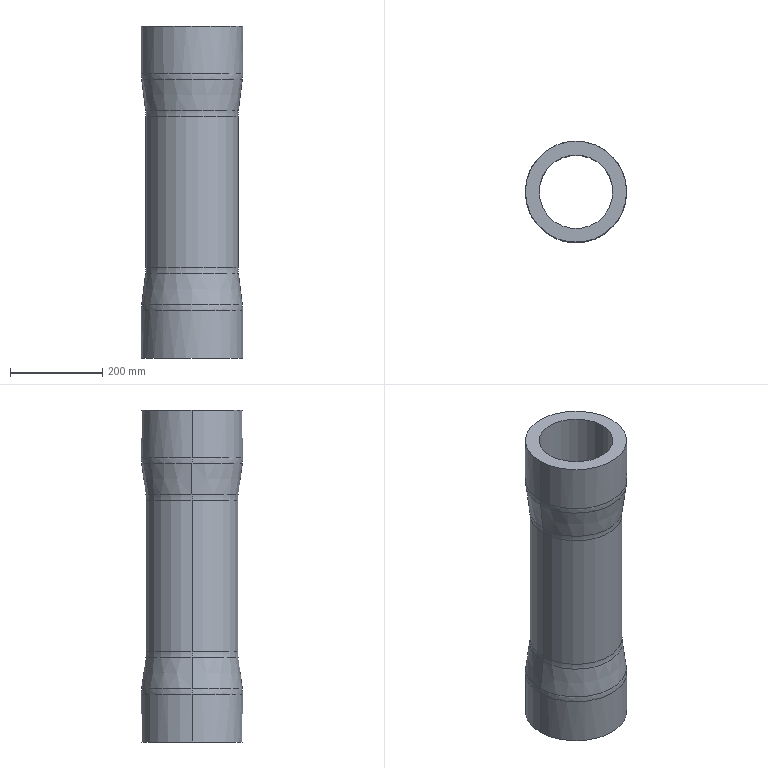Part | NX | features BREP 1 | 1 solid | 22 faces | box 220 x 220 x 721 mm | volume 10125039 mm3 | torus 8 | cylinder 8 | cone 4 | plane 2 | commonest cylinder face diameters 220 x4 160 x2 200 x2
STEP:
#1=CARTESIAN_POINT('',(0.,109.228,604.822));
#2=VERTEX_POINT('',#1);
#3=CARTESIAN_POINT('',(-109.228,0.000000027,604.822));
#4=VERTEX_POINT('',#3);
#5=CARTESIAN_POINT('',(0.,109.227,604.822));
#6=CARTESIAN_POINT('',(-14.298,109.227,604.822));
#7=CARTESIAN_POINT('',(-42.887,103.54,604.822));
#8=CARTESIAN_POINT('',(-79.246,79.246,604.822));
#9=CARTESIAN_POINT('',(-103.54,42.887,604.822));
#10=CARTESIAN_POINT('',(-109.227,14.298,604.822));
#11=CARTESIAN_POINT('',(-109.227,0.000000027,604.822));
#12=B_SPLINE_CURVE_WITH_KNOTS('',3,(#5,#6,#7,#8,#9,#10,#11),.UNSPECIFIED.,.F.,.F.,(4,1,1,1,4),(0.,0.25,0.5,0.75,1.),.UNSPECIFIED.);
#13=EDGE_CURVE('',#2,#4,#12,.T.);
#14=ORIENTED_EDGE('',*,*,#13,.T.);
#15=CARTESIAN_POINT('',(-110.,0.,617.226));
#16=VERTEX_POINT('',#15);
#17=CARTESIAN_POINT('',(-10.,0.,617.226));
#18=DIRECTION('',(0.,-1.,0.));
#19=DIRECTION('',(-1.,0.,0.));
#20=AXIS2_PLACEMENT_3D('',#17,#18,#19);
#21=CIRCLE('',#20,100.);
#22=EDGE_CURVE('',#16,#4,#21,.T.);
#23=ORIENTED_EDGE('',*,*,#22,.F.);
#24=CARTESIAN_POINT('',(0.,110.,617.226));
#25=VERTEX_POINT('',#24);
#26=CARTESIAN_POINT('',(0.,110.,617.226));
#27=CARTESIAN_POINT('',(-14.399,110.,617.226));
#28=CARTESIAN_POINT('',(-43.19,104.272,617.226));
#29=CARTESIAN_POINT('',(-79.807,79.807,617.226));
#30=CARTESIAN_POINT('',(-104.272,43.19,617.226));
#31=CARTESIAN_POINT('',(-110.,14.399,617.226));
#32=CARTESIAN_POINT('',(-110.,0.,617.226));
#33=B_SPLINE_CURVE_WITH_KNOTS('',3,(#26,#27,#28,#29,#30,#31,#32),.UNSPECIFIED.,.F.,.F.,(4,1,1,1,4),(0.,0.25,0.5,0.75,1.),.UNSPECIFIED.);
#34=EDGE_CURVE('',#16,#25,#33,.F.);
#35=ORIENTED_EDGE('',*,*,#34,.T.);
#36=CARTESIAN_POINT('',(110.,0.,617.226));
#37=VERTEX_POINT('',#36);
#38=CARTESIAN_POINT('',(110.,0.,617.226));
#39=CARTESIAN_POINT('',(110.,14.399,617.226));
#40=CARTESIAN_POINT('',(104.272,43.19,617.226));
#41=CARTESIAN_POINT('',(79.807,79.807,617.226));
#42=CARTESIAN_POINT('',(43.19,104.272,617.226));
#43=CARTESIAN_POINT('',(14.399,110.,617.226));
#44=CARTESIAN_POINT('',(0.,110.,617.226));
#45=B_SPLINE_CURVE_WITH_KNOTS('',3,(#38,#39,#40,#41,#42,#43,#44),.UNSPECIFIED.,.F.,.F.,(4,1,1,1,4),(0.,0.25,0.5,0.75,1.),.UNSPECIFIED.);
#46=EDGE_CURVE('',#25,#37,#45,.F.);
#47=ORIENTED_EDGE('',*,*,#46,.T.);
#48=CARTESIAN_POINT('',(109.228,0.000000027,604.822));
#49=VERTEX_POINT('',#48);
#50=CARTESIAN_POINT('',(10.,0.,617.226));
#51=DIRECTION('',(0.,1.,0.));
#52=DIRECTION('',(1.,0.,0.));
#53=AXIS2_PLACEMENT_3D('',#50,#51,#52);
#54=CIRCLE('',#53,100.);
#55=EDGE_CURVE('',#37,#49,#54,.T.);
#56=ORIENTED_EDGE('',*,*,#55,.T.);
#57=CARTESIAN_POINT('',(109.227,0.000000027,604.822));
#58=CARTESIAN_POINT('',(109.227,14.298,604.822));
#59=CARTESIAN_POINT('',(103.54,42.887,604.822));
#60=CARTESIAN_POINT('',(79.246,79.246,604.822));
#61=CARTESIAN_POINT('',(42.887,103.54,604.822));
#62=CARTESIAN_POINT('',(14.298,109.227,604.822));
#63=CARTESIAN_POINT('',(0.,109.227,604.822));
#64=B_SPLINE_CURVE_WITH_KNOTS('',3,(#57,#58,#59,#60,#61,#62,#63),.UNSPECIFIED.,.F.,.F.,(4,1,1,1,4),(0.,0.25,0.5,0.75,1.),.UNSPECIFIED.);
#65=EDGE_CURVE('',#49,#2,#64,.T.);
#66=ORIENTED_EDGE('',*,*,#65,.T.);
#67=EDGE_LOOP('',(#14,#23,#35,#47,#56,#66));
#68=FACE_BOUND('',#67,.T.);
#69=CARTESIAN_POINT('',(0.,0.,617.226));
#70=DIRECTION('',(0.,0.,1.));
#71=DIRECTION('',(0.,-1.,0.));
#72=AXIS2_PLACEMENT_3D('',#69,#70,#71);
#73=DEGENERATE_TOROIDAL_SURFACE('',#72,10.,100.,.T.);
#74=ADVANCED_FACE('',(#68),#73,.T.);
#75=CARTESIAN_POINT('',(-100.772,0.,537.178));
#76=VERTEX_POINT('',#75);
#77=CARTESIAN_POINT('',(-109.228,0.,604.822));
#78=CARTESIAN_POINT('',(-106.409,0.,582.274));
#79=CARTESIAN_POINT('',(-103.591,0.,559.726));
#80=CARTESIAN_POINT('',(-100.772,0.,537.178));
#81=B_SPLINE_CURVE_WITH_KNOTS('',3,(#77,#78,#79,#80),.UNSPECIFIED.,.F.,.F.,(4,4),(0.,1.),.UNSPECIFIED.);
#82=EDGE_CURVE('',#4,#76,#81,.T.);
#83=ORIENTED_EDGE('',*,*,#82,.F.);
#84=ORIENTED_EDGE('',*,*,#13,.F.);
#85=ORIENTED_EDGE('',*,*,#65,.F.);
#86=CARTESIAN_POINT('',(100.772,0.,537.178));
#87=VERTEX_POINT('',#86);
#88=CARTESIAN_POINT('',(109.228,0.,604.822));
#89=CARTESIAN_POINT('',(106.409,0.,582.274));
#90=CARTESIAN_POINT('',(103.591,0.,559.726));
#91=CARTESIAN_POINT('',(100.772,0.,537.178));
#92=B_SPLINE_CURVE_WITH_KNOTS('',3,(#88,#89,#90,#91),.UNSPECIFIED.,.F.,.F.,(4,4),(0.,1.),.UNSPECIFIED.);
#93=EDGE_CURVE('',#49,#87,#92,.T.);
#94=ORIENTED_EDGE('',*,*,#93,.T.);
#95=CARTESIAN_POINT('',(0.,0.,537.178));
#96=DIRECTION('',(0.,0.,-1.));
#97=DIRECTION('',(-1.,0.,0.));
#98=AXIS2_PLACEMENT_3D('',#95,#96,#97);
#99=CIRCLE('',#98,100.772);
#100=EDGE_CURVE('',#76,#87,#99,.T.);
#101=ORIENTED_EDGE('',*,*,#100,.F.);
#102=EDGE_LOOP('',(#83,#84,#85,#94,#101));
#103=FACE_BOUND('',#102,.T.);
#104=CARTESIAN_POINT('',(0.,0.,571.));
#105=DIRECTION('',(0.,0.,1.));
#106=DIRECTION('',(1.,0.,0.));
#107=AXIS2_PLACEMENT_3D('',#104,#105,#106);
#108=CONICAL_SURFACE('',#107,105.,0.1244);
#109=ADVANCED_FACE('',(#103),#108,.T.);
#110=CARTESIAN_POINT('',(100.,0.,524.774));
#111=VERTEX_POINT('',#110);
#112=CARTESIAN_POINT('',(-100.,0.,524.774));
#113=VERTEX_POINT('',#112);
#114=CARTESIAN_POINT('',(0.,0.,524.774));
#115=DIRECTION('',(0.,0.,1.));
#116=DIRECTION('',(1.,0.,0.));
#117=AXIS2_PLACEMENT_3D('',#114,#115,#116);
#118=CIRCLE('',#117,100.);
#119=EDGE_CURVE('',#111,#113,#118,.T.);
#120=ORIENTED_EDGE('',*,*,#119,.T.);
#121=CARTESIAN_POINT('',(-200.,0.,524.774));
#122=DIRECTION('',(0.,1.,0.));
#123=DIRECTION('',(0.9923,0.,0.124));
#124=AXIS2_PLACEMENT_3D('',#121,#122,#123);
#125=CIRCLE('',#124,100.);
#126=EDGE_CURVE('',#76,#113,#125,.T.);
#127=ORIENTED_EDGE('',*,*,#126,.F.);
#128=ORIENTED_EDGE('',*,*,#100,.T.);
#129=CARTESIAN_POINT('',(200.,0.,524.774));
#130=DIRECTION('',(0.,-1.,0.));
#131=DIRECTION('',(-0.9923,0.,0.124));
#132=AXIS2_PLACEMENT_3D('',#129,#130,#131);
#133=CIRCLE('',#132,100.);
#134=EDGE_CURVE('',#87,#111,#133,.T.);
#135=ORIENTED_EDGE('',*,*,#134,.T.);
#136=EDGE_LOOP('',(#120,#127,#128,#135));
#137=FACE_BOUND('',#136,.T.);
#138=CARTESIAN_POINT('',(0.,0.,524.774));
#139=DIRECTION('',(0.,0.,-1.));
#140=DIRECTION('',(-1.,0.,0.));
#141=AXIS2_PLACEMENT_3D('',#138,#139,#140);
#142=TOROIDAL_SURFACE('',#141,200.,100.);
#143=ADVANCED_FACE('',(#137),#142,.F.);
#144=ORIENTED_EDGE('',*,*,#134,.F.);
#145=CARTESIAN_POINT('',(0.,0.,537.178));
#146=DIRECTION('',(0.,0.,-1.));
#147=DIRECTION('',(1.,0.,0.));
#148=AXIS2_PLACEMENT_3D('',#145,#146,#147);
#149=CIRCLE('',#148,100.772);
#150=EDGE_CURVE('',#87,#76,#149,.T.);
#151=ORIENTED_EDGE('',*,*,#150,.T.);
#152=ORIENTED_EDGE('',*,*,#126,.T.);
#153=CARTESIAN_POINT('',(0.,0.,524.774));
#154=DIRECTION('',(0.,0.,1.));
#155=DIRECTION('',(-1.,0.,0.));
#156=AXIS2_PLACEMENT_3D('',#153,#154,#155);
#157=CIRCLE('',#156,100.);
#158=EDGE_CURVE('',#113,#111,#157,.T.);
#159=ORIENTED_EDGE('',*,*,#158,.T.);
#160=EDGE_LOOP('',(#144,#151,#152,#159));
#161=FACE_BOUND('',#160,.T.);
#162=CARTESIAN_POINT('',(0.,0.,524.774));
#163=DIRECTION('',(0.,0.,-1.));
#164=DIRECTION('',(1.,0.,0.));
#165=AXIS2_PLACEMENT_3D('',#162,#163,#164);
#166=TOROIDAL_SURFACE('',#165,200.,100.);
#167=ADVANCED_FACE('',(#161),#166,.F.);
#168=ORIENTED_EDGE('',*,*,#158,.F.);
#169=CARTESIAN_POINT('',(-100.,0.,196.226));
#170=VERTEX_POINT('',#169);
#171=CARTESIAN_POINT('',(-100.,0.,196.226));
#172=DIRECTION('',(0.,0.,1.));
#173=VECTOR('',#172,1000.);
#174=LINE('',#171,#173);
#175=EDGE_CURVE('',#170,#113,#174,.T.);
#176=ORIENTED_EDGE('',*,*,#175,.F.);
#177=CARTESIAN_POINT('',(100.,0.,196.226));
#178=VERTEX_POINT('',#177);
#179=CARTESIAN_POINT('',(0.,0.,196.226));
#180=DIRECTION('',(0.,0.,-1.));
#181=DIRECTION('',(1.,0.,0.));
#182=AXIS2_PLACEMENT_3D('',#179,#180,#181);
#183=CIRCLE('',#182,100.);
#184=EDGE_CURVE('',#178,#170,#183,.T.);
#185=ORIENTED_EDGE('',*,*,#184,.F.);
#186=CARTESIAN_POINT('',(100.,0.,196.226));
#187=DIRECTION('',(0.,0.,1.));
#188=VECTOR('',#187,1000.);
#189=LINE('',#186,#188);
#190=EDGE_CURVE('',#178,#111,#189,.T.);
#191=ORIENTED_EDGE('',*,*,#190,.T.);
#192=EDGE_LOOP('',(#168,#176,#185,#191));
#193=FACE_BOUND('',#192,.T.);
#194=CARTESIAN_POINT('',(0.,0.,-36.05));
#195=DIRECTION('',(0.,0.,-1.));
#196=DIRECTION('',(-1.,0.,0.));
#197=AXIS2_PLACEMENT_3D('',#194,#195,#196);
#198=CYLINDRICAL_SURFACE('',#197,100.);
#199=ADVANCED_FACE('',(#193),#198,.T.);
#200=ORIENTED_EDGE('',*,*,#190,.F.);
#201=CARTESIAN_POINT('',(0.,0.,196.226));
#202=DIRECTION('',(0.,0.,-1.));
#203=DIRECTION('',(-1.,0.,0.));
#204=AXIS2_PLACEMENT_3D('',#201,#202,#203);
#205=CIRCLE('',#204,100.);
#206=EDGE_CURVE('',#170,#178,#205,.T.);
#207=ORIENTED_EDGE('',*,*,#206,.F.);
#208=ORIENTED_EDGE('',*,*,#175,.T.);
#209=ORIENTED_EDGE('',*,*,#119,.F.);
#210=EDGE_LOOP('',(#200,#207,#208,#209));
#211=FACE_BOUND('',#210,.T.);
#212=CARTESIAN_POINT('',(0.,0.,-36.05));
#213=DIRECTION('',(0.,0.,-1.));
#214=DIRECTION('',(-1.,0.,0.));
#215=AXIS2_PLACEMENT_3D('',#212,#213,#214);
#216=CYLINDRICAL_SURFACE('',#215,100.);
#217=ADVANCED_FACE('',(#211),#216,.T.);
#218=CARTESIAN_POINT('',(100.772,0.,183.822));
#219=VERTEX_POINT('',#218);
#220=CARTESIAN_POINT('',(-100.772,0.,183.822));
#221=VERTEX_POINT('',#220);
#222=CARTESIAN_POINT('',(0.,0.,183.822));
#223=DIRECTION('',(0.,0.,1.));
#224=DIRECTION('',(1.,0.,0.));
#225=AXIS2_PLACEMENT_3D('',#222,#223,#224);
#226=CIRCLE('',#225,100.772);
#227=EDGE_CURVE('',#219,#221,#226,.T.);
#228=ORIENTED_EDGE('',*,*,#227,.T.);
#229=CARTESIAN_POINT('',(-200.,0.,196.226));
#230=DIRECTION('',(0.,1.,0.));
#231=DIRECTION('',(1.,0.,0.));
#232=AXIS2_PLACEMENT_3D('',#229,#230,#231);
#233=CIRCLE('',#232,100.);
#234=EDGE_CURVE('',#170,#221,#233,.T.);
#235=ORIENTED_EDGE('',*,*,#234,.F.);
#236=ORIENTED_EDGE('',*,*,#206,.T.);
#237=CARTESIAN_POINT('',(200.,0.,196.226));
#238=DIRECTION('',(0.,-1.,0.));
#239=DIRECTION('',(-1.,0.,0.));
#240=AXIS2_PLACEMENT_3D('',#237,#238,#239);
#241=CIRCLE('',#240,100.);
#242=EDGE_CURVE('',#178,#219,#241,.T.);
#243=ORIENTED_EDGE('',*,*,#242,.T.);
#244=EDGE_LOOP('',(#228,#235,#236,#243));
#245=FACE_BOUND('',#244,.T.);
#246=CARTESIAN_POINT('',(0.,0.,196.226));
#247=DIRECTION('',(0.,0.,-1.));
#248=DIRECTION('',(-1.,0.,0.));
#249=AXIS2_PLACEMENT_3D('',#246,#247,#248);
#250=TOROIDAL_SURFACE('',#249,200.,100.);
#251=ADVANCED_FACE('',(#245),#250,.F.);
#252=ORIENTED_EDGE('',*,*,#242,.F.);
#253=ORIENTED_EDGE('',*,*,#184,.T.);
#254=ORIENTED_EDGE('',*,*,#234,.T.);
#255=CARTESIAN_POINT('',(0.,0.,183.822));
#256=DIRECTION('',(0.,0.,1.));
#257=DIRECTION('',(-1.,0.,0.));
#258=AXIS2_PLACEMENT_3D('',#255,#256,#257);
#259=CIRCLE('',#258,100.772);
#260=EDGE_CURVE('',#221,#219,#259,.T.);
#261=ORIENTED_EDGE('',*,*,#260,.T.);
#262=EDGE_LOOP('',(#252,#253,#254,#261));
#263=FACE_BOUND('',#262,.T.);
#264=CARTESIAN_POINT('',(0.,0.,196.226));
#265=DIRECTION('',(0.,0.,-1.));
#266=DIRECTION('',(1.,0.,0.));
#267=AXIS2_PLACEMENT_3D('',#264,#265,#266);
#268=TOROIDAL_SURFACE('',#267,200.,100.);
#269=ADVANCED_FACE('',(#263),#268,.F.);
#270=ORIENTED_EDGE('',*,*,#260,.F.);
#271=CARTESIAN_POINT('',(-109.228,-0.000000027,116.178));
#272=VERTEX_POINT('',#271);
#273=CARTESIAN_POINT('',(-109.228,0.,116.178));
#274=CARTESIAN_POINT('',(-106.409,0.,138.726));
#275=CARTESIAN_POINT('',(-103.591,0.,161.274));
#276=CARTESIAN_POINT('',(-100.772,0.,183.822));
#277=B_SPLINE_CURVE_WITH_KNOTS('',3,(#273,#274,#275,#276),.UNSPECIFIED.,.F.,.F.,(4,4),(0.,1.),.UNSPECIFIED.);
#278=EDGE_CURVE('',#272,#221,#277,.T.);
#279=ORIENTED_EDGE('',*,*,#278,.F.);
#280=CARTESIAN_POINT('',(0.,-109.228,116.178));
#281=VERTEX_POINT('',#280);
#282=CARTESIAN_POINT('',(0.,-109.227,116.178));
#283=CARTESIAN_POINT('',(-14.298,-109.227,116.178));
#284=CARTESIAN_POINT('',(-42.887,-103.54,116.178));
#285=CARTESIAN_POINT('',(-79.246,-79.246,116.178));
#286=CARTESIAN_POINT('',(-103.54,-42.887,116.178));
#287=CARTESIAN_POINT('',(-109.227,-14.298,116.178));
#288=CARTESIAN_POINT('',(-109.227,-0.000000027,116.178));
#289=B_SPLINE_CURVE_WITH_KNOTS('',3,(#282,#283,#284,#285,#286,#287,#288),.UNSPECIFIED.,.F.,.F.,(4,1,1,1,4),(0.,0.25,0.5,0.75,1.),.UNSPECIFIED.);
#290=EDGE_CURVE('',#281,#272,#289,.T.);
#291=ORIENTED_EDGE('',*,*,#290,.F.);
#292=CARTESIAN_POINT('',(109.228,0.,116.178));
#293=VERTEX_POINT('',#292);
#294=CARTESIAN_POINT('',(109.227,0.,116.178));
#295=CARTESIAN_POINT('',(109.227,-14.298,116.178));
#296=CARTESIAN_POINT('',(103.54,-42.887,116.178));
#297=CARTESIAN_POINT('',(79.246,-79.246,116.178));
#298=CARTESIAN_POINT('',(42.887,-103.54,116.178));
#299=CARTESIAN_POINT('',(14.298,-109.227,116.178));
#300=CARTESIAN_POINT('',(0.,-109.227,116.178));
#301=B_SPLINE_CURVE_WITH_KNOTS('',3,(#294,#295,#296,#297,#298,#299,#300),.UNSPECIFIED.,.F.,.F.,(4,1,1,1,4),(0.,0.25,0.5,0.75,1.),.UNSPECIFIED.);
#302=EDGE_CURVE('',#293,#281,#301,.T.);
#303=ORIENTED_EDGE('',*,*,#302,.F.);
#304=CARTESIAN_POINT('',(109.228,0.,116.178));
#305=CARTESIAN_POINT('',(106.409,0.,138.726));
#306=CARTESIAN_POINT('',(103.591,0.,161.274));
#307=CARTESIAN_POINT('',(100.772,0.,183.822));
#308=B_SPLINE_CURVE_WITH_KNOTS('',3,(#304,#305,#306,#307),.UNSPECIFIED.,.F.,.F.,(4,4),(0.,1.),.UNSPECIFIED.);
#309=EDGE_CURVE('',#293,#219,#308,.T.);
#310=ORIENTED_EDGE('',*,*,#309,.T.);
#311=EDGE_LOOP('',(#270,#279,#291,#303,#310));
#312=FACE_BOUND('',#311,.T.);
#313=CARTESIAN_POINT('',(0.,0.,150.));
#314=DIRECTION('',(0.,0.,-1.));
#315=DIRECTION('',(-1.,0.,0.));
#316=AXIS2_PLACEMENT_3D('',#313,#314,#315);
#317=CONICAL_SURFACE('',#316,105.,0.1244);
#318=ADVANCED_FACE('',(#312),#317,.T.);
#319=ORIENTED_EDGE('',*,*,#309,.F.);
#320=CARTESIAN_POINT('',(0.,109.228,116.178));
#321=VERTEX_POINT('',#320);
#322=CARTESIAN_POINT('',(0.,109.227,116.178));
#323=CARTESIAN_POINT('',(14.298,109.227,116.178));
#324=CARTESIAN_POINT('',(42.887,103.54,116.178));
#325=CARTESIAN_POINT('',(79.246,79.246,116.178));
#326=CARTESIAN_POINT('',(103.54,42.887,116.178));
#327=CARTESIAN_POINT('',(109.227,14.298,116.178));
#328=CARTESIAN_POINT('',(109.227,0.,116.178));
#329=B_SPLINE_CURVE_WITH_KNOTS('',3,(#322,#323,#324,#325,#326,#327,#328),.UNSPECIFIED.,.F.,.F.,(4,1,1,1,4),(0.,0.25,0.5,0.75,1.),.UNSPECIFIED.);
#330=EDGE_CURVE('',#321,#293,#329,.T.);
#331=ORIENTED_EDGE('',*,*,#330,.F.);
#332=CARTESIAN_POINT('',(-109.227,-0.000000027,116.178));
#333=CARTESIAN_POINT('',(-109.227,14.298,116.178));
#334=CARTESIAN_POINT('',(-103.54,42.887,116.178));
#335=CARTESIAN_POINT('',(-79.246,79.246,116.178));
#336=CARTESIAN_POINT('',(-42.887,103.54,116.178));
#337=CARTESIAN_POINT('',(-14.298,109.227,116.178));
#338=CARTESIAN_POINT('',(0.,109.227,116.178));
#339=B_SPLINE_CURVE_WITH_KNOTS('',3,(#332,#333,#334,#335,#336,#337,#338),.UNSPECIFIED.,.F.,.F.,(4,1,1,1,4),(0.,0.25,0.5,0.75,1.),.UNSPECIFIED.);
#340=EDGE_CURVE('',#272,#321,#339,.T.);
#341=ORIENTED_EDGE('',*,*,#340,.F.);
#342=ORIENTED_EDGE('',*,*,#278,.T.);
#343=ORIENTED_EDGE('',*,*,#227,.F.);
#344=EDGE_LOOP('',(#319,#331,#341,#342,#343));
#345=FACE_BOUND('',#344,.T.);
#346=CARTESIAN_POINT('',(0.,0.,150.));
#347=DIRECTION('',(0.,0.,-1.));
#348=DIRECTION('',(-1.,0.,0.));
#349=AXIS2_PLACEMENT_3D('',#346,#347,#348);
#350=CONICAL_SURFACE('',#349,105.,0.1244);
#351=ADVANCED_FACE('',(#345),#350,.T.);
#352=CARTESIAN_POINT('',(0.,110.,103.774));
#353=VERTEX_POINT('',#352);
#354=CARTESIAN_POINT('',(-110.,0.,103.774));
#355=VERTEX_POINT('',#354);
#356=CARTESIAN_POINT('',(-110.,0.,103.774));
#357=CARTESIAN_POINT('',(-110.,14.399,103.774));
#358=CARTESIAN_POINT('',(-104.272,43.19,103.774));
#359=CARTESIAN_POINT('',(-79.807,79.807,103.774));
#360=CARTESIAN_POINT('',(-43.19,104.272,103.774));
#361=CARTESIAN_POINT('',(-14.399,110.,103.774));
#362=CARTESIAN_POINT('',(0.,110.,103.774));
#363=B_SPLINE_CURVE_WITH_KNOTS('',3,(#356,#357,#358,#359,#360,#361,#362),.UNSPECIFIED.,.F.,.F.,(4,1,1,1,4),(0.,0.25,0.5,0.75,1.),.UNSPECIFIED.);
#364=EDGE_CURVE('',#353,#355,#363,.F.);
#365=ORIENTED_EDGE('',*,*,#364,.T.);
#366=CARTESIAN_POINT('',(-10.,0.,103.774));
#367=DIRECTION('',(0.,-1.,0.));
#368=DIRECTION('',(-0.9923,0.,0.124));
#369=AXIS2_PLACEMENT_3D('',#366,#367,#368);
#370=CIRCLE('',#369,100.);
#371=EDGE_CURVE('',#272,#355,#370,.T.);
#372=ORIENTED_EDGE('',*,*,#371,.F.);
#373=ORIENTED_EDGE('',*,*,#340,.T.);
#374=ORIENTED_EDGE('',*,*,#330,.T.);
#375=CARTESIAN_POINT('',(110.,0.,103.774));
#376=VERTEX_POINT('',#375);
#377=CARTESIAN_POINT('',(10.,0.,103.774));
#378=DIRECTION('',(0.,1.,0.));
#379=DIRECTION('',(0.9923,0.,0.124));
#380=AXIS2_PLACEMENT_3D('',#377,#378,#379);
#381=CIRCLE('',#380,100.);
#382=EDGE_CURVE('',#293,#376,#381,.T.);
#383=ORIENTED_EDGE('',*,*,#382,.T.);
#384=CARTESIAN_POINT('',(0.,110.,103.774));
#385=CARTESIAN_POINT('',(14.399,110.,103.774));
#386=CARTESIAN_POINT('',(43.19,104.272,103.774));
#387=CARTESIAN_POINT('',(79.807,79.807,103.774));
#388=CARTESIAN_POINT('',(104.272,43.19,103.774));
#389=CARTESIAN_POINT('',(110.,14.399,103.774));
#390=CARTESIAN_POINT('',(110.,0.,103.774));
#391=B_SPLINE_CURVE_WITH_KNOTS('',3,(#384,#385,#386,#387,#388,#389,#390),.UNSPECIFIED.,.F.,.F.,(4,1,1,1,4),(0.,0.25,0.5,0.75,1.),.UNSPECIFIED.);
#392=EDGE_CURVE('',#376,#353,#391,.F.);
#393=ORIENTED_EDGE('',*,*,#392,.T.);
#394=EDGE_LOOP('',(#365,#372,#373,#374,#383,#393));
#395=FACE_BOUND('',#394,.T.);
#396=CARTESIAN_POINT('',(0.,0.,103.774));
#397=DIRECTION('',(0.,0.,1.));
#398=DIRECTION('',(0.,-1.,0.));
#399=AXIS2_PLACEMENT_3D('',#396,#397,#398);
#400=DEGENERATE_TOROIDAL_SURFACE('',#399,10.,100.,.T.);
#401=ADVANCED_FACE('',(#395),#400,.T.);
#402=ORIENTED_EDGE('',*,*,#392,.F.);
#403=CARTESIAN_POINT('',(110.,0.,0.));
#404=VERTEX_POINT('',#403);
#405=CARTESIAN_POINT('',(110.,0.,0.));
#406=CARTESIAN_POINT('',(110.,0.,34.591));
#407=CARTESIAN_POINT('',(110.,0.,69.183));
#408=CARTESIAN_POINT('',(110.,0.,103.774));
#409=B_SPLINE_CURVE_WITH_KNOTS('',3,(#405,#406,#407,#408),.UNSPECIFIED.,.F.,.F.,(4,4),(0.,1.),.UNSPECIFIED.);
#410=EDGE_CURVE('',#376,#404,#409,.F.);
#411=ORIENTED_EDGE('',*,*,#410,.T.);
#412=CARTESIAN_POINT('',(-110.,0.,0.));
#413=VERTEX_POINT('',#412);
#414=CARTESIAN_POINT('',(0.,0.,0.));
#415=DIRECTION('',(0.,0.,-1.));
#416=DIRECTION('',(-1.,0.,0.));
#417=AXIS2_PLACEMENT_3D('',#414,#415,#416);
#418=CIRCLE('',#417,110.);
#419=EDGE_CURVE('',#413,#404,#418,.T.);
#420=ORIENTED_EDGE('',*,*,#419,.F.);
#421=CARTESIAN_POINT('',(-110.,0.,0.));
#422=CARTESIAN_POINT('',(-110.,0.,34.591));
#423=CARTESIAN_POINT('',(-110.,0.,69.183));
#424=CARTESIAN_POINT('',(-110.,0.,103.774));
#425=B_SPLINE_CURVE_WITH_KNOTS('',3,(#421,#422,#423,#424),.UNSPECIFIED.,.F.,.F.,(4,4),(0.,1.),.UNSPECIFIED.);
#426=EDGE_CURVE('',#355,#413,#425,.F.);
#427=ORIENTED_EDGE('',*,*,#426,.F.);
#428=ORIENTED_EDGE('',*,*,#364,.F.);
#429=EDGE_LOOP('',(#402,#411,#420,#427,#428));
#430=FACE_BOUND('',#429,.T.);
#431=CARTESIAN_POINT('',(0.,0.,721.));
#432=DIRECTION('',(0.,0.,-1.));
#433=DIRECTION('',(-1.,0.,0.));
#434=AXIS2_PLACEMENT_3D('',#431,#432,#433);
#435=CYLINDRICAL_SURFACE('',#434,110.);
#436=ADVANCED_FACE('',(#430),#435,.T.);
#437=CARTESIAN_POINT('',(0.,-110.,103.774));
#438=VERTEX_POINT('',#437);
#439=CARTESIAN_POINT('',(110.,0.,103.774));
#440=CARTESIAN_POINT('',(110.,-14.399,103.774));
#441=CARTESIAN_POINT('',(104.272,-43.19,103.774));
#442=CARTESIAN_POINT('',(79.807,-79.807,103.774));
#443=CARTESIAN_POINT('',(43.19,-104.272,103.774));
#444=CARTESIAN_POINT('',(14.399,-110.,103.774));
#445=CARTESIAN_POINT('',(0.,-110.,103.774));
#446=B_SPLINE_CURVE_WITH_KNOTS('',3,(#439,#440,#441,#442,#443,#444,#445),.UNSPECIFIED.,.F.,.F.,(4,1,1,1,4),(0.,0.25,0.5,0.75,1.),.UNSPECIFIED.);
#447=EDGE_CURVE('',#438,#376,#446,.F.);
#448=ORIENTED_EDGE('',*,*,#447,.F.);
#449=CARTESIAN_POINT('',(0.,-110.,103.774));
#450=CARTESIAN_POINT('',(-14.399,-110.,103.774));
#451=CARTESIAN_POINT('',(-43.19,-104.272,103.774));
#452=CARTESIAN_POINT('',(-79.807,-79.807,103.774));
#453=CARTESIAN_POINT('',(-104.272,-43.19,103.774));
#454=CARTESIAN_POINT('',(-110.,-14.399,103.774));
#455=CARTESIAN_POINT('',(-110.,0.,103.774));
#456=B_SPLINE_CURVE_WITH_KNOTS('',3,(#449,#450,#451,#452,#453,#454,#455),.UNSPECIFIED.,.F.,.F.,(4,1,1,1,4),(0.,0.25,0.5,0.75,1.),.UNSPECIFIED.);
#457=EDGE_CURVE('',#355,#438,#456,.F.);
#458=ORIENTED_EDGE('',*,*,#457,.F.);
#459=ORIENTED_EDGE('',*,*,#426,.T.);
#460=CARTESIAN_POINT('',(0.,0.,0.));
#461=DIRECTION('',(0.,0.,-1.));
#462=DIRECTION('',(1.,0.,0.));
#463=AXIS2_PLACEMENT_3D('',#460,#461,#462);
#464=CIRCLE('',#463,110.);
#465=EDGE_CURVE('',#404,#413,#464,.T.);
#466=ORIENTED_EDGE('',*,*,#465,.F.);
#467=ORIENTED_EDGE('',*,*,#410,.F.);
#468=EDGE_LOOP('',(#448,#458,#459,#466,#467));
#469=FACE_BOUND('',#468,.T.);
#470=CARTESIAN_POINT('',(0.,0.,721.));
#471=DIRECTION('',(0.,0.,-1.));
#472=DIRECTION('',(-1.,0.,0.));
#473=AXIS2_PLACEMENT_3D('',#470,#471,#472);
#474=CYLINDRICAL_SURFACE('',#473,110.);
#475=ADVANCED_FACE('',(#469),#474,.T.);
#476=ORIENTED_EDGE('',*,*,#419,.T.);
#477=ORIENTED_EDGE('',*,*,#465,.T.);
#478=EDGE_LOOP('',(#476,#477));
#479=FACE_BOUND('',#478,.T.);
#480=CARTESIAN_POINT('',(-80.,0.,0.));
#481=VERTEX_POINT('',#480);
#482=CARTESIAN_POINT('',(80.,0.,0.));
#483=VERTEX_POINT('',#482);
#484=CARTESIAN_POINT('',(0.,0.,0.));
#485=DIRECTION('',(0.,0.,1.));
#486=DIRECTION('',(-1.,0.,0.));
#487=AXIS2_PLACEMENT_3D('',#484,#485,#486);
#488=CIRCLE('',#487,80.);
#489=EDGE_CURVE('',#481,#483,#488,.T.);
#490=ORIENTED_EDGE('',*,*,#489,.T.);
#491=CARTESIAN_POINT('',(0.,0.,0.));
#492=DIRECTION('',(0.,0.,1.));
#493=DIRECTION('',(1.,0.,0.));
#494=AXIS2_PLACEMENT_3D('',#491,#492,#493);
#495=CIRCLE('',#494,80.);
#496=EDGE_CURVE('',#483,#481,#495,.T.);
#497=ORIENTED_EDGE('',*,*,#496,.T.);
#498=EDGE_LOOP('',(#490,#497));
#499=FACE_BOUND('',#498,.T.);
#500=CARTESIAN_POINT('',(0.,0.,0.));
#501=DIRECTION('',(0.,0.,1.));
#502=DIRECTION('',(1.,0.,0.));
#503=AXIS2_PLACEMENT_3D('',#500,#501,#502);
#504=PLANE('',#503);
#505=ADVANCED_FACE('',(#479,#499),#504,.F.);
#506=ORIENTED_EDGE('',*,*,#496,.F.);
#507=CARTESIAN_POINT('',(80.,0.,721.));
#508=VERTEX_POINT('',#507);
#509=CARTESIAN_POINT('',(80.,0.,721.));
#510=DIRECTION('',(0.,0.,-1.));
#511=VECTOR('',#510,1000.);
#512=LINE('',#509,#511);
#513=EDGE_CURVE('',#483,#508,#512,.F.);
#514=ORIENTED_EDGE('',*,*,#513,.T.);
#515=CARTESIAN_POINT('',(-80.,0.,721.));
#516=VERTEX_POINT('',#515);
#517=CARTESIAN_POINT('',(0.,0.,721.));
#518=DIRECTION('',(0.,0.,-1.));
#519=DIRECTION('',(-1.,0.,0.));
#520=AXIS2_PLACEMENT_3D('',#517,#518,#519);
#521=CIRCLE('',#520,80.);
#522=EDGE_CURVE('',#516,#508,#521,.T.);
#523=ORIENTED_EDGE('',*,*,#522,.F.);
#524=CARTESIAN_POINT('',(-80.,0.,721.));
#525=DIRECTION('',(0.,0.,-1.));
#526=VECTOR('',#525,1000.);
#527=LINE('',#524,#526);
#528=EDGE_CURVE('',#481,#516,#527,.F.);
#529=ORIENTED_EDGE('',*,*,#528,.F.);
#530=EDGE_LOOP('',(#506,#514,#523,#529));
#531=FACE_BOUND('',#530,.T.);
#532=CARTESIAN_POINT('',(0.,0.,0.));
#533=DIRECTION('',(0.,0.,1.));
#534=DIRECTION('',(1.,0.,0.));
#535=AXIS2_PLACEMENT_3D('',#532,#533,#534);
#536=CYLINDRICAL_SURFACE('',#535,80.);
#537=ADVANCED_FACE('',(#531),#536,.F.);
#538=ORIENTED_EDGE('',*,*,#528,.T.);
#539=CARTESIAN_POINT('',(0.,0.,721.));
#540=DIRECTION('',(0.,0.,-1.));
#541=DIRECTION('',(1.,0.,0.));
#542=AXIS2_PLACEMENT_3D('',#539,#540,#541);
#543=CIRCLE('',#542,80.);
#544=EDGE_CURVE('',#508,#516,#543,.T.);
#545=ORIENTED_EDGE('',*,*,#544,.F.);
#546=ORIENTED_EDGE('',*,*,#513,.F.);
#547=ORIENTED_EDGE('',*,*,#489,.F.);
#548=EDGE_LOOP('',(#538,#545,#546,#547));
#549=FACE_BOUND('',#548,.T.);
#550=CARTESIAN_POINT('',(0.,0.,0.));
#551=DIRECTION('',(0.,0.,1.));
#552=DIRECTION('',(1.,0.,0.));
#553=AXIS2_PLACEMENT_3D('',#550,#551,#552);
#554=CYLINDRICAL_SURFACE('',#553,80.);
#555=ADVANCED_FACE('',(#549),#554,.F.);
#556=CARTESIAN_POINT('',(110.,0.,721.));
#557=VERTEX_POINT('',#556);
#558=CARTESIAN_POINT('',(-110.,0.,721.));
#559=VERTEX_POINT('',#558);
#560=CARTESIAN_POINT('',(0.,0.,721.));
#561=DIRECTION('',(0.,0.,1.));
#562=DIRECTION('',(1.,0.,0.));
#563=AXIS2_PLACEMENT_3D('',#560,#561,#562);
#564=CIRCLE('',#563,110.);
#565=EDGE_CURVE('',#557,#559,#564,.T.);
#566=ORIENTED_EDGE('',*,*,#565,.T.);
#567=CARTESIAN_POINT('',(0.,0.,721.));
#568=DIRECTION('',(0.,0.,1.));
#569=DIRECTION('',(-1.,0.,0.));
#570=AXIS2_PLACEMENT_3D('',#567,#568,#569);
#571=CIRCLE('',#570,110.);
#572=EDGE_CURVE('',#559,#557,#571,.T.);
#573=ORIENTED_EDGE('',*,*,#572,.T.);
#574=EDGE_LOOP('',(#566,#573));
#575=FACE_BOUND('',#574,.T.);
#576=ORIENTED_EDGE('',*,*,#544,.T.);
#577=ORIENTED_EDGE('',*,*,#522,.T.);
#578=EDGE_LOOP('',(#576,#577));
#579=FACE_BOUND('',#578,.T.);
#580=CARTESIAN_POINT('',(0.,0.,721.));
#581=DIRECTION('',(0.,0.,1.));
#582=DIRECTION('',(1.,0.,0.));
#583=AXIS2_PLACEMENT_3D('',#580,#581,#582);
#584=PLANE('',#583);
#585=ADVANCED_FACE('',(#575,#579),#584,.T.);
#586=ORIENTED_EDGE('',*,*,#572,.F.);
#587=CARTESIAN_POINT('',(-110.,0.,617.226));
#588=CARTESIAN_POINT('',(-110.,0.,651.817));
#589=CARTESIAN_POINT('',(-110.,0.,686.409));
#590=CARTESIAN_POINT('',(-110.,0.,721.));
#591=B_SPLINE_CURVE_WITH_KNOTS('',3,(#587,#588,#589,#590),.UNSPECIFIED.,.F.,.F.,(4,4),(0.000000002,1.),.UNSPECIFIED.);
#592=EDGE_CURVE('',#16,#559,#591,.T.);
#593=ORIENTED_EDGE('',*,*,#592,.F.);
#594=CARTESIAN_POINT('',(0.,-110.,617.226));
#595=VERTEX_POINT('',#594);
#596=CARTESIAN_POINT('',(-110.,0.,617.226));
#597=CARTESIAN_POINT('',(-110.,-14.399,617.226));
#598=CARTESIAN_POINT('',(-104.272,-43.19,617.226));
#599=CARTESIAN_POINT('',(-79.807,-79.807,617.226));
#600=CARTESIAN_POINT('',(-43.19,-104.272,617.226));
#601=CARTESIAN_POINT('',(-14.399,-110.,617.226));
#602=CARTESIAN_POINT('',(0.,-110.,617.226));
#603=B_SPLINE_CURVE_WITH_KNOTS('',3,(#596,#597,#598,#599,#600,#601,#602),.UNSPECIFIED.,.F.,.F.,(4,1,1,1,4),(0.,0.25,0.5,0.75,1.),.UNSPECIFIED.);
#604=EDGE_CURVE('',#595,#16,#603,.F.);
#605=ORIENTED_EDGE('',*,*,#604,.F.);
#606=CARTESIAN_POINT('',(0.,-110.,617.226));
#607=CARTESIAN_POINT('',(14.399,-110.,617.226));
#608=CARTESIAN_POINT('',(43.19,-104.272,617.226));
#609=CARTESIAN_POINT('',(79.807,-79.807,617.226));
#610=CARTESIAN_POINT('',(104.272,-43.19,617.226));
#611=CARTESIAN_POINT('',(110.,-14.399,617.226));
#612=CARTESIAN_POINT('',(110.,0.,617.226));
#613=B_SPLINE_CURVE_WITH_KNOTS('',3,(#606,#607,#608,#609,#610,#611,#612),.UNSPECIFIED.,.F.,.F.,(4,1,1,1,4),(0.,0.25,0.5,0.75,1.),.UNSPECIFIED.);
#614=EDGE_CURVE('',#37,#595,#613,.F.);
#615=ORIENTED_EDGE('',*,*,#614,.F.);
#616=CARTESIAN_POINT('',(110.,0.,617.226));
#617=CARTESIAN_POINT('',(110.,0.,651.817));
#618=CARTESIAN_POINT('',(110.,0.,686.409));
#619=CARTESIAN_POINT('',(110.,0.,721.));
#620=B_SPLINE_CURVE_WITH_KNOTS('',3,(#616,#617,#618,#619),.UNSPECIFIED.,.F.,.F.,(4,4),(0.000000002,1.),.UNSPECIFIED.);
#621=EDGE_CURVE('',#37,#557,#620,.T.);
#622=ORIENTED_EDGE('',*,*,#621,.T.);
#623=EDGE_LOOP('',(#586,#593,#605,#615,#622));
#624=FACE_BOUND('',#623,.T.);
#625=CARTESIAN_POINT('',(0.,0.,721.));
#626=DIRECTION('',(0.,0.,-1.));
#627=DIRECTION('',(-1.,0.,0.));
#628=AXIS2_PLACEMENT_3D('',#625,#626,#627);
#629=CYLINDRICAL_SURFACE('',#628,110.);
#630=ADVANCED_FACE('',(#624),#629,.T.);
#631=ORIENTED_EDGE('',*,*,#621,.F.);
#632=ORIENTED_EDGE('',*,*,#46,.F.);
#633=ORIENTED_EDGE('',*,*,#34,.F.);
#634=ORIENTED_EDGE('',*,*,#592,.T.);
#635=ORIENTED_EDGE('',*,*,#565,.F.);
#636=EDGE_LOOP('',(#631,#632,#633,#634,#635));
#637=FACE_BOUND('',#636,.T.);
#638=CARTESIAN_POINT('',(0.,0.,721.));
#639=DIRECTION('',(0.,0.,-1.));
#640=DIRECTION('',(-1.,0.,0.));
#641=AXIS2_PLACEMENT_3D('',#638,#639,#640);
#642=CYLINDRICAL_SURFACE('',#641,110.);
#643=ADVANCED_FACE('',(#637),#642,.T.);
#644=CARTESIAN_POINT('',(0.,-109.228,604.822));
#645=VERTEX_POINT('',#644);
#646=CARTESIAN_POINT('',(-109.227,0.000000027,604.822));
#647=CARTESIAN_POINT('',(-109.227,-14.298,604.822));
#648=CARTESIAN_POINT('',(-103.54,-42.887,604.822));
#649=CARTESIAN_POINT('',(-79.246,-79.246,604.822));
#650=CARTESIAN_POINT('',(-42.887,-103.54,604.822));
#651=CARTESIAN_POINT('',(-14.298,-109.227,604.822));
#652=CARTESIAN_POINT('',(0.,-109.227,604.822));
#653=B_SPLINE_CURVE_WITH_KNOTS('',3,(#646,#647,#648,#649,#650,#651,#652),.UNSPECIFIED.,.F.,.F.,(4,1,1,1,4),(0.,0.25,0.5,0.75,1.),.UNSPECIFIED.);
#654=EDGE_CURVE('',#4,#645,#653,.T.);
#655=ORIENTED_EDGE('',*,*,#654,.T.);
#656=CARTESIAN_POINT('',(0.,-109.227,604.822));
#657=CARTESIAN_POINT('',(14.298,-109.227,604.822));
#658=CARTESIAN_POINT('',(42.887,-103.54,604.822));
#659=CARTESIAN_POINT('',(79.246,-79.246,604.822));
#660=CARTESIAN_POINT('',(103.54,-42.887,604.822));
#661=CARTESIAN_POINT('',(109.227,-14.298,604.822));
#662=CARTESIAN_POINT('',(109.227,0.000000027,604.822));
#663=B_SPLINE_CURVE_WITH_KNOTS('',3,(#656,#657,#658,#659,#660,#661,#662),.UNSPECIFIED.,.F.,.F.,(4,1,1,1,4),(0.,0.25,0.5,0.75,1.),.UNSPECIFIED.);
#664=EDGE_CURVE('',#645,#49,#663,.T.);
#665=ORIENTED_EDGE('',*,*,#664,.T.);
#666=ORIENTED_EDGE('',*,*,#55,.F.);
#667=ORIENTED_EDGE('',*,*,#614,.T.);
#668=ORIENTED_EDGE('',*,*,#604,.T.);
#669=ORIENTED_EDGE('',*,*,#22,.T.);
#670=EDGE_LOOP('',(#655,#665,#666,#667,#668,#669));
#671=FACE_BOUND('',#670,.T.);
#672=CARTESIAN_POINT('',(0.,0.,617.226));
#673=DIRECTION('',(0.,0.,1.));
#674=DIRECTION('',(0.,-1.,0.));
#675=AXIS2_PLACEMENT_3D('',#672,#673,#674);
#676=DEGENERATE_TOROIDAL_SURFACE('',#675,10.,100.,.T.);
#677=ADVANCED_FACE('',(#671),#676,.T.);
#678=ORIENTED_EDGE('',*,*,#150,.F.);
#679=ORIENTED_EDGE('',*,*,#93,.F.);
#680=ORIENTED_EDGE('',*,*,#664,.F.);
#681=ORIENTED_EDGE('',*,*,#654,.F.);
#682=ORIENTED_EDGE('',*,*,#82,.T.);
#683=EDGE_LOOP('',(#678,#679,#680,#681,#682));
#684=FACE_BOUND('',#683,.T.);
#685=CARTESIAN_POINT('',(0.,0.,571.));
#686=DIRECTION('',(0.,0.,1.));
#687=DIRECTION('',(1.,0.,0.));
#688=AXIS2_PLACEMENT_3D('',#685,#686,#687);
#689=CONICAL_SURFACE('',#688,105.,0.1244);
#690=ADVANCED_FACE('',(#684),#689,.T.);
#691=ORIENTED_EDGE('',*,*,#457,.T.);
#692=ORIENTED_EDGE('',*,*,#447,.T.);
#693=ORIENTED_EDGE('',*,*,#382,.F.);
#694=ORIENTED_EDGE('',*,*,#302,.T.);
#695=ORIENTED_EDGE('',*,*,#290,.T.);
#696=ORIENTED_EDGE('',*,*,#371,.T.);
#697=EDGE_LOOP('',(#691,#692,#693,#694,#695,#696));
#698=FACE_BOUND('',#697,.T.);
#699=CARTESIAN_POINT('',(0.,0.,103.774));
#700=DIRECTION('',(0.,0.,1.));
#701=DIRECTION('',(0.,-1.,0.));
#702=AXIS2_PLACEMENT_3D('',#699,#700,#701);
#703=DEGENERATE_TOROIDAL_SURFACE('',#702,10.,100.,.T.);
#704=ADVANCED_FACE('',(#698),#703,.T.);
#705=CLOSED_SHELL('',(#74,#109,#143,#167,#199,#217,#251,#269,#318,#351,#401,#436,#475,#505,#537,#555,#585,#630,#643,#677,#690,#704));
#706=MANIFOLD_SOLID_BREP('',#705);
#707=(LENGTH_UNIT()NAMED_UNIT(*)SI_UNIT(.MILLI.,.METRE.));
#708=UNCERTAINTY_MEASURE_WITH_UNIT(LENGTH_MEASURE(0.0508),#707,'','');
#709=(NAMED_UNIT(*)PLANE_ANGLE_UNIT()SI_UNIT($,.RADIAN.));
#710=(NAMED_UNIT(*)SI_UNIT($,.STERADIAN.)SOLID_ANGLE_UNIT());
#711=(GEOMETRIC_REPRESENTATION_CONTEXT(3)GLOBAL_UNCERTAINTY_ASSIGNED_CONTEXT((#708))GLOBAL_UNIT_ASSIGNED_CONTEXT((#707,#709,#710))REPRESENTATION_CONTEXT('',''));
#712=ADVANCED_BREP_SHAPE_REPRESENTATION('',(#706),#711);